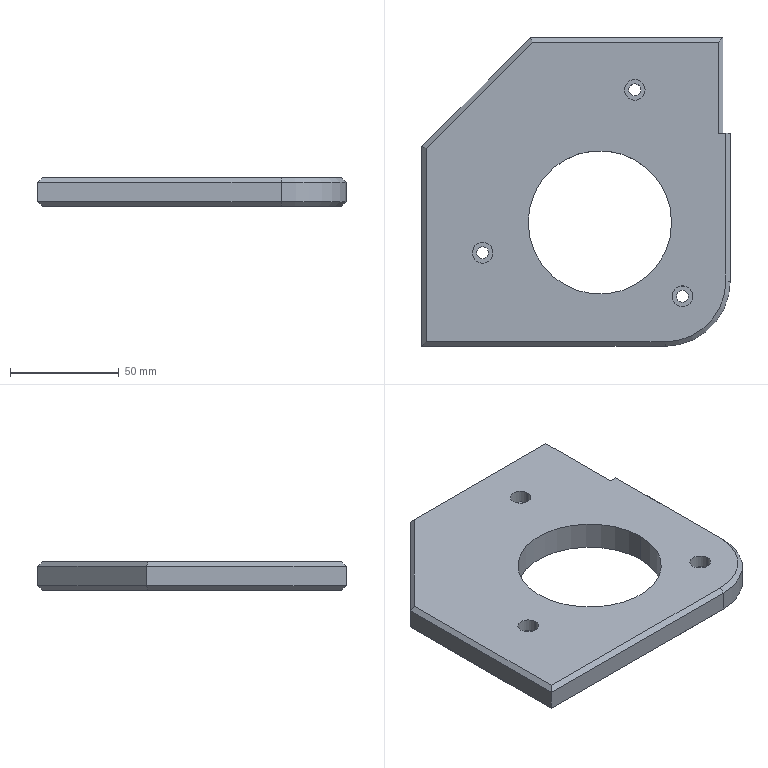Part | Creo | 1 solid | 41 faces | box 142 x 142 x 13 mm | volume 193049 mm3 | plane 24 | cylinder 15 | cone 2 | commonest cylinder face diameters 5.5 x6 9.5 x6 66 x2 60 x1
STEP:
#1=CARTESIAN_POINT('',(-313.,234.995,-24.));
#2=VERTEX_POINT('',#1);
#3=CARTESIAN_POINT('',(-203.,234.995,-24.));
#4=VERTEX_POINT('',#3);
#5=CARTESIAN_POINT('',(-313.,234.995,-24.));
#6=DIRECTION('',(1.,0.,0.));
#7=VECTOR('',#6,110.);
#8=LINE('',#5,#7);
#9=EDGE_CURVE('',#2,#4,#8,.T.);
#10=ORIENTED_EDGE('',*,*,#9,.T.);
#11=CARTESIAN_POINT('',(-175.,262.995,-24.));
#12=VERTEX_POINT('',#11);
#13=CARTESIAN_POINT('',(-203.,262.995,-24.));
#14=DIRECTION('',(0.,0.,-1.));
#15=DIRECTION('',(1.,0.,0.));
#16=AXIS2_PLACEMENT_3D('',#13,#14,#15);
#17=CIRCLE('',#16,28.);
#18=EDGE_CURVE('',#12,#4,#17,.T.);
#19=ORIENTED_EDGE('',*,*,#18,.F.);
#20=CARTESIAN_POINT('',(-175.,330.995,-24.));
#21=VERTEX_POINT('',#20);
#22=CARTESIAN_POINT('',(-175.,262.995,-24.));
#23=DIRECTION('',(0.,1.,0.));
#24=VECTOR('',#23,68.);
#25=LINE('',#22,#24);
#26=EDGE_CURVE('',#12,#21,#25,.T.);
#27=ORIENTED_EDGE('',*,*,#26,.T.);
#28=CARTESIAN_POINT('',(-178.5,330.995,-24.));
#29=VERTEX_POINT('',#28);
#30=CARTESIAN_POINT('',(-175.,330.995,-24.));
#31=DIRECTION('',(-1.,0.,0.));
#32=VECTOR('',#31,3.5);
#33=LINE('',#30,#32);
#34=EDGE_CURVE('',#21,#29,#33,.T.);
#35=ORIENTED_EDGE('',*,*,#34,.T.);
#36=CARTESIAN_POINT('',(-178.5,372.995,-24.));
#37=VERTEX_POINT('',#36);
#38=CARTESIAN_POINT('',(-178.5,330.995,-24.));
#39=DIRECTION('',(0.,1.,0.));
#40=VECTOR('',#39,42.);
#41=LINE('',#38,#40);
#42=EDGE_CURVE('',#29,#37,#41,.T.);
#43=ORIENTED_EDGE('',*,*,#42,.T.);
#44=CARTESIAN_POINT('',(-264.172,372.995,-24.));
#45=VERTEX_POINT('',#44);
#46=CARTESIAN_POINT('',(-178.5,372.995,-24.));
#47=DIRECTION('',(-1.,0.,0.));
#48=VECTOR('',#47,85.672);
#49=LINE('',#46,#48);
#50=EDGE_CURVE('',#37,#45,#49,.T.);
#51=ORIENTED_EDGE('',*,*,#50,.T.);
#52=CARTESIAN_POINT('',(-313.,324.167,-24.));
#53=VERTEX_POINT('',#52);
#54=CARTESIAN_POINT('',(-313.,324.167,-24.));
#55=DIRECTION('',(0.7071,0.7071,0.));
#56=VECTOR('',#55,69.054);
#57=LINE('',#54,#56);
#58=EDGE_CURVE('',#53,#45,#57,.T.);
#59=ORIENTED_EDGE('',*,*,#58,.F.);
#60=CARTESIAN_POINT('',(-313.,324.167,-24.));
#61=DIRECTION('',(0.,-1.,0.));
#62=VECTOR('',#61,89.172);
#63=LINE('',#60,#62);
#64=EDGE_CURVE('',#53,#2,#63,.T.);
#65=ORIENTED_EDGE('',*,*,#64,.T.);
#66=EDGE_LOOP('',(#10,#19,#27,#35,#43,#51,#59,#65));
#67=FACE_OUTER_BOUND('',#66,.F.);
#68=CARTESIAN_POINT('',(-289.75,276.,-24.));
#69=VERTEX_POINT('',#68);
#70=CARTESIAN_POINT('',(-284.25,276.,-24.));
#71=VERTEX_POINT('',#70);
#72=CARTESIAN_POINT('',(-287.,276.,-24.));
#73=DIRECTION('',(0.,0.,1.));
#74=DIRECTION('',(-1.,0.,0.));
#75=AXIS2_PLACEMENT_3D('',#72,#73,#74);
#76=CIRCLE('',#75,2.75);
#77=EDGE_CURVE('',#69,#71,#76,.T.);
#78=ORIENTED_EDGE('',*,*,#77,.F.);
#79=CARTESIAN_POINT('',(-287.,276.,-24.));
#80=DIRECTION('',(0.,0.,1.));
#81=DIRECTION('',(1.,0.,0.));
#82=AXIS2_PLACEMENT_3D('',#79,#80,#81);
#83=CIRCLE('',#82,2.75);
#84=EDGE_CURVE('',#71,#69,#83,.T.);
#85=ORIENTED_EDGE('',*,*,#84,.F.);
#86=EDGE_LOOP('',(#78,#85));
#87=FACE_BOUND('',#86,.F.);
#88=CARTESIAN_POINT('',(-219.699,351.,-24.));
#89=VERTEX_POINT('',#88);
#90=CARTESIAN_POINT('',(-214.199,351.,-24.));
#91=VERTEX_POINT('',#90);
#92=CARTESIAN_POINT('',(-216.949,351.,-24.));
#93=DIRECTION('',(0.,0.,1.));
#94=DIRECTION('',(-1.,0.,0.));
#95=AXIS2_PLACEMENT_3D('',#92,#93,#94);
#96=CIRCLE('',#95,2.75);
#97=EDGE_CURVE('',#89,#91,#96,.T.);
#98=ORIENTED_EDGE('',*,*,#97,.F.);
#99=CARTESIAN_POINT('',(-216.949,351.,-24.));
#100=DIRECTION('',(0.,0.,1.));
#101=DIRECTION('',(1.,0.,0.));
#102=AXIS2_PLACEMENT_3D('',#99,#100,#101);
#103=CIRCLE('',#102,2.75);
#104=EDGE_CURVE('',#91,#89,#103,.T.);
#105=ORIENTED_EDGE('',*,*,#104,.F.);
#106=EDGE_LOOP('',(#98,#105));
#107=FACE_BOUND('',#106,.F.);
#108=CARTESIAN_POINT('',(-197.75,256.,-24.));
#109=VERTEX_POINT('',#108);
#110=CARTESIAN_POINT('',(-192.25,256.,-24.));
#111=VERTEX_POINT('',#110);
#112=CARTESIAN_POINT('',(-195.,256.,-24.));
#113=DIRECTION('',(0.,0.,1.));
#114=DIRECTION('',(-1.,0.,0.));
#115=AXIS2_PLACEMENT_3D('',#112,#113,#114);
#116=CIRCLE('',#115,2.75);
#117=EDGE_CURVE('',#109,#111,#116,.T.);
#118=ORIENTED_EDGE('',*,*,#117,.F.);
#119=CARTESIAN_POINT('',(-195.,256.,-24.));
#120=DIRECTION('',(0.,0.,1.));
#121=DIRECTION('',(1.,0.,0.));
#122=AXIS2_PLACEMENT_3D('',#119,#120,#121);
#123=CIRCLE('',#122,2.75);
#124=EDGE_CURVE('',#111,#109,#123,.T.);
#125=ORIENTED_EDGE('',*,*,#124,.F.);
#126=EDGE_LOOP('',(#118,#125));
#127=FACE_BOUND('',#126,.F.);
#128=CARTESIAN_POINT('',(-266.,289.995,-24.));
#129=VERTEX_POINT('',#128);
#130=CARTESIAN_POINT('',(-200.,289.995,-24.));
#131=VERTEX_POINT('',#130);
#132=CARTESIAN_POINT('',(-233.,289.995,-24.));
#133=DIRECTION('',(0.,0.,1.));
#134=DIRECTION('',(-1.,0.,0.));
#135=AXIS2_PLACEMENT_3D('',#132,#133,#134);
#136=CIRCLE('',#135,33.);
#137=EDGE_CURVE('',#129,#131,#136,.T.);
#138=ORIENTED_EDGE('',*,*,#137,.F.);
#139=CARTESIAN_POINT('',(-233.,289.995,-24.));
#140=DIRECTION('',(0.,0.,1.));
#141=DIRECTION('',(1.,0.,0.));
#142=AXIS2_PLACEMENT_3D('',#139,#140,#141);
#143=CIRCLE('',#142,33.);
#144=EDGE_CURVE('',#131,#129,#143,.T.);
#145=ORIENTED_EDGE('',*,*,#144,.F.);
#146=EDGE_LOOP('',(#138,#145));
#147=FACE_BOUND('',#146,.F.);
#148=CARTESIAN_POINT('',(-223.,300.495,-24.));
#149=DIRECTION('',(0.,0.,-1.));
#150=DIRECTION('',(-1.,0.,0.));
#151=AXIS2_PLACEMENT_3D('',#148,#149,#150);
#152=PLANE('',#151);
#153=ADVANCED_FACE('',(#67,#87,#107,#127,#147),#152,.T.);
#154=ORIENTED_EDGE('',*,*,#117,.T.);
#155=CARTESIAN_POINT('',(-192.25,256.,-17.));
#156=VERTEX_POINT('',#155);
#157=CARTESIAN_POINT('',(-192.25,256.,-24.));
#158=DIRECTION('',(0.,0.,1.));
#159=VECTOR('',#158,7.);
#160=LINE('',#157,#159);
#161=EDGE_CURVE('',#111,#156,#160,.T.);
#162=ORIENTED_EDGE('',*,*,#161,.T.);
#163=CARTESIAN_POINT('',(-197.75,256.,-17.));
#164=VERTEX_POINT('',#163);
#165=CARTESIAN_POINT('',(-195.,256.,-17.));
#166=DIRECTION('',(0.,0.,-1.));
#167=DIRECTION('',(1.,0.,0.));
#168=AXIS2_PLACEMENT_3D('',#165,#166,#167);
#169=CIRCLE('',#168,2.75);
#170=EDGE_CURVE('',#156,#164,#169,.T.);
#171=ORIENTED_EDGE('',*,*,#170,.T.);
#172=CARTESIAN_POINT('',(-197.75,256.,-24.));
#173=DIRECTION('',(0.,0.,1.));
#174=VECTOR('',#173,7.);
#175=LINE('',#172,#174);
#176=EDGE_CURVE('',#109,#164,#175,.T.);
#177=ORIENTED_EDGE('',*,*,#176,.F.);
#178=EDGE_LOOP('',(#154,#162,#171,#177));
#179=FACE_OUTER_BOUND('',#178,.F.);
#180=CARTESIAN_POINT('',(-195.,256.,-11.));
#181=DIRECTION('',(0.,0.,1.));
#182=DIRECTION('',(1.,0.,0.));
#183=AXIS2_PLACEMENT_3D('',#180,#181,#182);
#184=CYLINDRICAL_SURFACE('',#183,2.75);
#185=ADVANCED_FACE('',(#179),#184,.F.);
#186=ORIENTED_EDGE('',*,*,#124,.T.);
#187=ORIENTED_EDGE('',*,*,#176,.T.);
#188=CARTESIAN_POINT('',(-195.,256.,-17.));
#189=DIRECTION('',(0.,0.,-1.));
#190=DIRECTION('',(-1.,0.,0.));
#191=AXIS2_PLACEMENT_3D('',#188,#189,#190);
#192=CIRCLE('',#191,2.75);
#193=EDGE_CURVE('',#164,#156,#192,.T.);
#194=ORIENTED_EDGE('',*,*,#193,.T.);
#195=ORIENTED_EDGE('',*,*,#161,.F.);
#196=EDGE_LOOP('',(#186,#187,#194,#195));
#197=FACE_OUTER_BOUND('',#196,.F.);
#198=CARTESIAN_POINT('',(-195.,256.,-11.));
#199=DIRECTION('',(0.,0.,1.));
#200=DIRECTION('',(1.,0.,0.));
#201=AXIS2_PLACEMENT_3D('',#198,#199,#200);
#202=CYLINDRICAL_SURFACE('',#201,2.75);
#203=ADVANCED_FACE('',(#197),#202,.F.);
#204=CARTESIAN_POINT('',(-190.25,256.,-17.));
#205=VERTEX_POINT('',#204);
#206=CARTESIAN_POINT('',(-199.75,256.,-17.));
#207=VERTEX_POINT('',#206);
#208=CARTESIAN_POINT('',(-195.,256.,-17.));
#209=DIRECTION('',(0.,0.,1.));
#210=DIRECTION('',(1.,0.,0.));
#211=AXIS2_PLACEMENT_3D('',#208,#209,#210);
#212=CIRCLE('',#211,4.75);
#213=EDGE_CURVE('',#205,#207,#212,.T.);
#214=ORIENTED_EDGE('',*,*,#213,.F.);
#215=CARTESIAN_POINT('',(-195.,256.,-17.));
#216=DIRECTION('',(0.,0.,1.));
#217=DIRECTION('',(-1.,0.,0.));
#218=AXIS2_PLACEMENT_3D('',#215,#216,#217);
#219=CIRCLE('',#218,4.75);
#220=EDGE_CURVE('',#207,#205,#219,.T.);
#221=ORIENTED_EDGE('',*,*,#220,.F.);
#222=EDGE_LOOP('',(#214,#221));
#223=FACE_OUTER_BOUND('',#222,.F.);
#224=ORIENTED_EDGE('',*,*,#170,.F.);
#225=ORIENTED_EDGE('',*,*,#193,.F.);
#226=EDGE_LOOP('',(#224,#225));
#227=FACE_BOUND('',#226,.F.);
#228=CARTESIAN_POINT('',(-195.,260.75,-17.));
#229=DIRECTION('',(0.,0.,-1.));
#230=DIRECTION('',(-1.,0.,0.));
#231=AXIS2_PLACEMENT_3D('',#228,#229,#230);
#232=PLANE('',#231);
#233=ADVANCED_FACE('',(#223,#227),#232,.F.);
#234=ORIENTED_EDGE('',*,*,#213,.T.);
#235=CARTESIAN_POINT('',(-199.75,256.,-11.));
#236=VERTEX_POINT('',#235);
#237=CARTESIAN_POINT('',(-199.75,256.,-17.));
#238=DIRECTION('',(0.,0.,1.));
#239=VECTOR('',#238,6.);
#240=LINE('',#237,#239);
#241=EDGE_CURVE('',#207,#236,#240,.T.);
#242=ORIENTED_EDGE('',*,*,#241,.T.);
#243=CARTESIAN_POINT('',(-190.25,256.,-11.));
#244=VERTEX_POINT('',#243);
#245=CARTESIAN_POINT('',(-195.,256.,-11.));
#246=DIRECTION('',(0.,0.,-1.));
#247=DIRECTION('',(-1.,0.,0.));
#248=AXIS2_PLACEMENT_3D('',#245,#246,#247);
#249=CIRCLE('',#248,4.75);
#250=EDGE_CURVE('',#236,#244,#249,.T.);
#251=ORIENTED_EDGE('',*,*,#250,.T.);
#252=CARTESIAN_POINT('',(-190.25,256.,-17.));
#253=DIRECTION('',(0.,0.,1.));
#254=VECTOR('',#253,6.);
#255=LINE('',#252,#254);
#256=EDGE_CURVE('',#205,#244,#255,.T.);
#257=ORIENTED_EDGE('',*,*,#256,.F.);
#258=EDGE_LOOP('',(#234,#242,#251,#257));
#259=FACE_OUTER_BOUND('',#258,.F.);
#260=CARTESIAN_POINT('',(-195.,256.,-11.));
#261=DIRECTION('',(0.,0.,1.));
#262=DIRECTION('',(1.,0.,0.));
#263=AXIS2_PLACEMENT_3D('',#260,#261,#262);
#264=CYLINDRICAL_SURFACE('',#263,4.75);
#265=ADVANCED_FACE('',(#259),#264,.F.);
#266=ORIENTED_EDGE('',*,*,#220,.T.);
#267=ORIENTED_EDGE('',*,*,#256,.T.);
#268=CARTESIAN_POINT('',(-195.,256.,-11.));
#269=DIRECTION('',(0.,0.,-1.));
#270=DIRECTION('',(1.,0.,0.));
#271=AXIS2_PLACEMENT_3D('',#268,#269,#270);
#272=CIRCLE('',#271,4.75);
#273=EDGE_CURVE('',#244,#236,#272,.T.);
#274=ORIENTED_EDGE('',*,*,#273,.T.);
#275=ORIENTED_EDGE('',*,*,#241,.F.);
#276=EDGE_LOOP('',(#266,#267,#274,#275));
#277=FACE_OUTER_BOUND('',#276,.F.);
#278=CARTESIAN_POINT('',(-195.,256.,-11.));
#279=DIRECTION('',(0.,0.,1.));
#280=DIRECTION('',(1.,0.,0.));
#281=AXIS2_PLACEMENT_3D('',#278,#279,#280);
#282=CYLINDRICAL_SURFACE('',#281,4.75);
#283=ADVANCED_FACE('',(#277),#282,.F.);
#284=CARTESIAN_POINT('',(-178.5,330.995,-11.));
#285=VERTEX_POINT('',#284);
#286=CARTESIAN_POINT('',(-175.,330.995,-11.));
#287=VERTEX_POINT('',#286);
#288=CARTESIAN_POINT('',(-178.5,330.995,-11.));
#289=DIRECTION('',(1.,0.,0.));
#290=VECTOR('',#289,3.5);
#291=LINE('',#288,#290);
#292=EDGE_CURVE('',#285,#287,#291,.T.);
#293=ORIENTED_EDGE('',*,*,#292,.T.);
#294=CARTESIAN_POINT('',(-175.,262.995,-11.));
#295=VERTEX_POINT('',#294);
#296=CARTESIAN_POINT('',(-175.,330.995,-11.));
#297=DIRECTION('',(0.,-1.,0.));
#298=VECTOR('',#297,68.);
#299=LINE('',#296,#298);
#300=EDGE_CURVE('',#287,#295,#299,.T.);
#301=ORIENTED_EDGE('',*,*,#300,.T.);
#302=CARTESIAN_POINT('',(-203.,234.995,-11.));
#303=VERTEX_POINT('',#302);
#304=CARTESIAN_POINT('',(-203.,262.995,-11.));
#305=DIRECTION('',(0.,0.,1.));
#306=DIRECTION('',(0.,-1.,0.));
#307=AXIS2_PLACEMENT_3D('',#304,#305,#306);
#308=CIRCLE('',#307,28.);
#309=EDGE_CURVE('',#303,#295,#308,.T.);
#310=ORIENTED_EDGE('',*,*,#309,.F.);
#311=CARTESIAN_POINT('',(-313.,234.995,-11.));
#312=VERTEX_POINT('',#311);
#313=CARTESIAN_POINT('',(-203.,234.995,-11.));
#314=DIRECTION('',(-1.,0.,0.));
#315=VECTOR('',#314,110.);
#316=LINE('',#313,#315);
#317=EDGE_CURVE('',#303,#312,#316,.T.);
#318=ORIENTED_EDGE('',*,*,#317,.T.);
#319=CARTESIAN_POINT('',(-313.,324.167,-11.));
#320=VERTEX_POINT('',#319);
#321=CARTESIAN_POINT('',(-313.,234.995,-11.));
#322=DIRECTION('',(0.,1.,0.));
#323=VECTOR('',#322,89.172);
#324=LINE('',#321,#323);
#325=EDGE_CURVE('',#312,#320,#324,.T.);
#326=ORIENTED_EDGE('',*,*,#325,.T.);
#327=CARTESIAN_POINT('',(-264.172,372.995,-11.));
#328=VERTEX_POINT('',#327);
#329=CARTESIAN_POINT('',(-264.172,372.995,-11.));
#330=DIRECTION('',(-0.7071,-0.7071,0.));
#331=VECTOR('',#330,69.054);
#332=LINE('',#329,#331);
#333=EDGE_CURVE('',#328,#320,#332,.T.);
#334=ORIENTED_EDGE('',*,*,#333,.F.);
#335=CARTESIAN_POINT('',(-178.5,372.995,-11.));
#336=VERTEX_POINT('',#335);
#337=CARTESIAN_POINT('',(-264.172,372.995,-11.));
#338=DIRECTION('',(1.,0.,0.));
#339=VECTOR('',#338,85.672);
#340=LINE('',#337,#339);
#341=EDGE_CURVE('',#328,#336,#340,.T.);
#342=ORIENTED_EDGE('',*,*,#341,.T.);
#343=CARTESIAN_POINT('',(-178.5,372.995,-11.));
#344=DIRECTION('',(0.,-1.,0.));
#345=VECTOR('',#344,42.);
#346=LINE('',#343,#345);
#347=EDGE_CURVE('',#336,#285,#346,.T.);
#348=ORIENTED_EDGE('',*,*,#347,.T.);
#349=EDGE_LOOP('',(#293,#301,#310,#318,#326,#334,#342,#348));
#350=FACE_OUTER_BOUND('',#349,.F.);
#351=ORIENTED_EDGE('',*,*,#273,.F.);
#352=ORIENTED_EDGE('',*,*,#250,.F.);
#353=EDGE_LOOP('',(#351,#352));
#354=FACE_BOUND('',#353,.F.);
#355=CARTESIAN_POINT('',(-282.25,276.,-11.));
#356=VERTEX_POINT('',#355);
#357=CARTESIAN_POINT('',(-291.75,276.,-11.));
#358=VERTEX_POINT('',#357);
#359=CARTESIAN_POINT('',(-287.,276.,-11.));
#360=DIRECTION('',(0.,0.,-1.));
#361=DIRECTION('',(1.,0.,0.));
#362=AXIS2_PLACEMENT_3D('',#359,#360,#361);
#363=CIRCLE('',#362,4.75);
#364=EDGE_CURVE('',#356,#358,#363,.T.);
#365=ORIENTED_EDGE('',*,*,#364,.F.);
#366=CARTESIAN_POINT('',(-287.,276.,-11.));
#367=DIRECTION('',(0.,0.,-1.));
#368=DIRECTION('',(-1.,0.,0.));
#369=AXIS2_PLACEMENT_3D('',#366,#367,#368);
#370=CIRCLE('',#369,4.75);
#371=EDGE_CURVE('',#358,#356,#370,.T.);
#372=ORIENTED_EDGE('',*,*,#371,.F.);
#373=EDGE_LOOP('',(#365,#372));
#374=FACE_BOUND('',#373,.F.);
#375=CARTESIAN_POINT('',(-212.199,351.,-11.));
#376=VERTEX_POINT('',#375);
#377=CARTESIAN_POINT('',(-221.699,351.,-11.));
#378=VERTEX_POINT('',#377);
#379=CARTESIAN_POINT('',(-216.949,351.,-11.));
#380=DIRECTION('',(0.,0.,-1.));
#381=DIRECTION('',(1.,0.,0.));
#382=AXIS2_PLACEMENT_3D('',#379,#380,#381);
#383=CIRCLE('',#382,4.75);
#384=EDGE_CURVE('',#376,#378,#383,.T.);
#385=ORIENTED_EDGE('',*,*,#384,.F.);
#386=CARTESIAN_POINT('',(-216.949,351.,-11.));
#387=DIRECTION('',(0.,0.,-1.));
#388=DIRECTION('',(-1.,0.,0.));
#389=AXIS2_PLACEMENT_3D('',#386,#387,#388);
#390=CIRCLE('',#389,4.75);
#391=EDGE_CURVE('',#378,#376,#390,.T.);
#392=ORIENTED_EDGE('',*,*,#391,.F.);
#393=EDGE_LOOP('',(#385,#392));
#394=FACE_BOUND('',#393,.F.);
#395=CARTESIAN_POINT('',(-200.,289.995,-11.));
#396=VERTEX_POINT('',#395);
#397=CARTESIAN_POINT('',(-266.,289.995,-11.));
#398=VERTEX_POINT('',#397);
#399=CARTESIAN_POINT('',(-233.,289.995,-11.));
#400=DIRECTION('',(0.,0.,-1.));
#401=DIRECTION('',(1.,0.,0.));
#402=AXIS2_PLACEMENT_3D('',#399,#400,#401);
#403=CIRCLE('',#402,33.);
#404=EDGE_CURVE('',#396,#398,#403,.T.);
#405=ORIENTED_EDGE('',*,*,#404,.F.);
#406=CARTESIAN_POINT('',(-233.,289.995,-11.));
#407=DIRECTION('',(0.,0.,-1.));
#408=DIRECTION('',(-1.,0.,0.));
#409=AXIS2_PLACEMENT_3D('',#406,#407,#408);
#410=CIRCLE('',#409,33.);
#411=EDGE_CURVE('',#398,#396,#410,.T.);
#412=ORIENTED_EDGE('',*,*,#411,.F.);
#413=EDGE_LOOP('',(#405,#412));
#414=FACE_BOUND('',#413,.F.);
#415=CARTESIAN_POINT('',(-223.,300.495,-11.));
#416=DIRECTION('',(0.,0.,1.));
#417=DIRECTION('',(1.,0.,0.));
#418=AXIS2_PLACEMENT_3D('',#415,#416,#417);
#419=PLANE('',#418);
#420=ADVANCED_FACE('',(#350,#354,#374,#394,#414),#419,.T.);
#421=CARTESIAN_POINT('',(-173.,330.995,-13.));
#422=VERTEX_POINT('',#421);
#423=CARTESIAN_POINT('',(-173.,330.995,-22.));
#424=VERTEX_POINT('',#423);
#425=CARTESIAN_POINT('',(-173.,330.995,-13.));
#426=DIRECTION('',(0.,0.,-1.));
#427=VECTOR('',#426,9.);
#428=LINE('',#425,#427);
#429=EDGE_CURVE('',#422,#424,#428,.T.);
#430=ORIENTED_EDGE('',*,*,#429,.F.);
#431=CARTESIAN_POINT('',(-175.,330.995,-11.));
#432=DIRECTION('',(0.7071,0.,-0.7071));
#433=VECTOR('',#432,2.828);
#434=LINE('',#431,#433);
#435=EDGE_CURVE('',#287,#422,#434,.T.);
#436=ORIENTED_EDGE('',*,*,#435,.F.);
#437=ORIENTED_EDGE('',*,*,#292,.F.);
#438=CARTESIAN_POINT('',(-176.5,330.995,-13.));
#439=VERTEX_POINT('',#438);
#440=CARTESIAN_POINT('',(-176.5,330.995,-13.));
#441=DIRECTION('',(-0.7071,0.,0.7071));
#442=VECTOR('',#441,2.828);
#443=LINE('',#440,#442);
#444=EDGE_CURVE('',#439,#285,#443,.T.);
#445=ORIENTED_EDGE('',*,*,#444,.F.);
#446=CARTESIAN_POINT('',(-176.5,330.995,-22.));
#447=VERTEX_POINT('',#446);
#448=CARTESIAN_POINT('',(-176.5,330.995,-13.));
#449=DIRECTION('',(0.,0.,-1.));
#450=VECTOR('',#449,9.);
#451=LINE('',#448,#450);
#452=EDGE_CURVE('',#439,#447,#451,.T.);
#453=ORIENTED_EDGE('',*,*,#452,.T.);
#454=CARTESIAN_POINT('',(-178.5,330.995,-24.));
#455=DIRECTION('',(0.7071,0.,0.7071));
#456=VECTOR('',#455,2.828);
#457=LINE('',#454,#456);
#458=EDGE_CURVE('',#29,#447,#457,.T.);
#459=ORIENTED_EDGE('',*,*,#458,.F.);
#460=ORIENTED_EDGE('',*,*,#34,.F.);
#461=CARTESIAN_POINT('',(-173.,330.995,-22.));
#462=DIRECTION('',(-0.7071,0.,-0.7071));
#463=VECTOR('',#462,2.828);
#464=LINE('',#461,#463);
#465=EDGE_CURVE('',#424,#21,#464,.T.);
#466=ORIENTED_EDGE('',*,*,#465,.F.);
#467=EDGE_LOOP('',(#430,#436,#437,#445,#453,#459,#460,#466));
#468=FACE_OUTER_BOUND('',#467,.F.);
#469=CARTESIAN_POINT('',(-155.,330.995,-1.));
#470=DIRECTION('',(0.,1.,0.));
#471=DIRECTION('',(-1.,0.,0.));
#472=AXIS2_PLACEMENT_3D('',#469,#470,#471);
#473=PLANE('',#472);
#474=ADVANCED_FACE('',(#468),#473,.T.);
#475=CARTESIAN_POINT('',(-173.,262.995,-22.));
#476=VERTEX_POINT('',#475);
#477=CARTESIAN_POINT('',(-173.,262.995,-13.));
#478=VERTEX_POINT('',#477);
#479=CARTESIAN_POINT('',(-173.,262.995,-22.));
#480=DIRECTION('',(0.,0.,1.));
#481=VECTOR('',#480,9.);
#482=LINE('',#479,#481);
#483=EDGE_CURVE('',#476,#478,#482,.T.);
#484=ORIENTED_EDGE('',*,*,#483,.T.);
#485=CARTESIAN_POINT('',(-173.,262.995,-13.));
#486=DIRECTION('',(0.,1.,0.));
#487=VECTOR('',#486,68.);
#488=LINE('',#485,#487);
#489=EDGE_CURVE('',#478,#422,#488,.T.);
#490=ORIENTED_EDGE('',*,*,#489,.T.);
#491=ORIENTED_EDGE('',*,*,#429,.T.);
#492=CARTESIAN_POINT('',(-173.,330.995,-22.));
#493=DIRECTION('',(0.,-1.,0.));
#494=VECTOR('',#493,68.);
#495=LINE('',#492,#494);
#496=EDGE_CURVE('',#424,#476,#495,.T.);
#497=ORIENTED_EDGE('',*,*,#496,.T.);
#498=EDGE_LOOP('',(#484,#490,#491,#497));
#499=FACE_OUTER_BOUND('',#498,.F.);
#500=CARTESIAN_POINT('',(-173.,-2.005,-23.));
#501=DIRECTION('',(-1.,0.,0.));
#502=DIRECTION('',(0.,1.,0.));
#503=AXIS2_PLACEMENT_3D('',#500,#501,#502);
#504=PLANE('',#503);
#505=ADVANCED_FACE('',(#499),#504,.F.);
#506=CARTESIAN_POINT('',(-203.,232.995,-13.));
#507=VERTEX_POINT('',#506);
#508=CARTESIAN_POINT('',(-203.,232.995,-22.));
#509=VERTEX_POINT('',#508);
#510=CARTESIAN_POINT('',(-203.,232.995,-13.));
#511=DIRECTION('',(0.,0.,-1.));
#512=VECTOR('',#511,9.);
#513=LINE('',#510,#512);
#514=EDGE_CURVE('',#507,#509,#513,.T.);
#515=ORIENTED_EDGE('',*,*,#514,.F.);
#516=CARTESIAN_POINT('',(-203.,262.995,-13.));
#517=DIRECTION('',(0.,0.,1.));
#518=DIRECTION('',(0.,-1.,0.));
#519=AXIS2_PLACEMENT_3D('',#516,#517,#518);
#520=CIRCLE('',#519,30.);
#521=EDGE_CURVE('',#507,#478,#520,.T.);
#522=ORIENTED_EDGE('',*,*,#521,.T.);
#523=ORIENTED_EDGE('',*,*,#483,.F.);
#524=CARTESIAN_POINT('',(-203.,262.995,-22.));
#525=DIRECTION('',(0.,0.,-1.));
#526=DIRECTION('',(1.,0.,0.));
#527=AXIS2_PLACEMENT_3D('',#524,#525,#526);
#528=CIRCLE('',#527,30.);
#529=EDGE_CURVE('',#476,#509,#528,.T.);
#530=ORIENTED_EDGE('',*,*,#529,.T.);
#531=EDGE_LOOP('',(#515,#522,#523,#530));
#532=FACE_OUTER_BOUND('',#531,.F.);
#533=CARTESIAN_POINT('',(-203.,262.995,-12.));
#534=DIRECTION('',(0.,0.,1.));
#535=DIRECTION('',(1.,0.,0.));
#536=AXIS2_PLACEMENT_3D('',#533,#534,#535);
#537=CYLINDRICAL_SURFACE('',#536,30.);
#538=ADVANCED_FACE('',(#532),#537,.T.);
#539=CARTESIAN_POINT('',(-315.,232.995,-22.));
#540=VERTEX_POINT('',#539);
#541=CARTESIAN_POINT('',(-315.,232.995,-13.));
#542=VERTEX_POINT('',#541);
#543=CARTESIAN_POINT('',(-315.,232.995,-22.));
#544=DIRECTION('',(0.,0.,1.));
#545=VECTOR('',#544,9.);
#546=LINE('',#543,#545);
#547=EDGE_CURVE('',#540,#542,#546,.T.);
#548=ORIENTED_EDGE('',*,*,#547,.T.);
#549=CARTESIAN_POINT('',(-315.,232.995,-13.));
#550=DIRECTION('',(1.,0.,0.));
#551=VECTOR('',#550,112.);
#552=LINE('',#549,#551);
#553=EDGE_CURVE('',#542,#507,#552,.T.);
#554=ORIENTED_EDGE('',*,*,#553,.T.);
#555=ORIENTED_EDGE('',*,*,#514,.T.);
#556=CARTESIAN_POINT('',(-203.,232.995,-22.));
#557=DIRECTION('',(-1.,0.,0.));
#558=VECTOR('',#557,112.);
#559=LINE('',#556,#558);
#560=EDGE_CURVE('',#509,#540,#559,.T.);
#561=ORIENTED_EDGE('',*,*,#560,.T.);
#562=EDGE_LOOP('',(#548,#554,#555,#561));
#563=FACE_OUTER_BOUND('',#562,.F.);
#564=CARTESIAN_POINT('',(-223.,232.995,-12.));
#565=DIRECTION('',(0.,-1.,0.));
#566=DIRECTION('',(0.,0.,-1.));
#567=AXIS2_PLACEMENT_3D('',#564,#565,#566);
#568=PLANE('',#567);
#569=ADVANCED_FACE('',(#563),#568,.T.);
#570=CARTESIAN_POINT('',(-315.,324.995,-22.));
#571=VERTEX_POINT('',#570);
#572=CARTESIAN_POINT('',(-315.,324.995,-13.));
#573=VERTEX_POINT('',#572);
#574=CARTESIAN_POINT('',(-315.,324.995,-22.));
#575=DIRECTION('',(0.,0.,1.));
#576=VECTOR('',#575,9.);
#577=LINE('',#574,#576);
#578=EDGE_CURVE('',#571,#573,#577,.T.);
#579=ORIENTED_EDGE('',*,*,#578,.T.);
#580=CARTESIAN_POINT('',(-315.,324.995,-13.));
#581=DIRECTION('',(0.,-1.,0.));
#582=VECTOR('',#581,92.);
#583=LINE('',#580,#582);
#584=EDGE_CURVE('',#573,#542,#583,.T.);
#585=ORIENTED_EDGE('',*,*,#584,.T.);
#586=ORIENTED_EDGE('',*,*,#547,.F.);
#587=CARTESIAN_POINT('',(-315.,232.995,-22.));
#588=DIRECTION('',(0.,1.,0.));
#589=VECTOR('',#588,92.);
#590=LINE('',#587,#589);
#591=EDGE_CURVE('',#540,#571,#590,.T.);
#592=ORIENTED_EDGE('',*,*,#591,.T.);
#593=EDGE_LOOP('',(#579,#585,#586,#592));
#594=FACE_OUTER_BOUND('',#593,.F.);
#595=CARTESIAN_POINT('',(-315.,-0.004699,-21.));
#596=DIRECTION('',(1.,0.,0.));
#597=DIRECTION('',(0.,-1.,0.));
#598=AXIS2_PLACEMENT_3D('',#595,#596,#597);
#599=PLANE('',#598);
#600=ADVANCED_FACE('',(#594),#599,.F.);
#601=CARTESIAN_POINT('',(-265.,374.995,-13.));
#602=VERTEX_POINT('',#601);
#603=CARTESIAN_POINT('',(-265.,374.995,-22.));
#604=VERTEX_POINT('',#603);
#605=CARTESIAN_POINT('',(-265.,374.995,-13.));
#606=DIRECTION('',(0.,0.,-1.));
#607=VECTOR('',#606,9.);
#608=LINE('',#605,#607);
#609=EDGE_CURVE('',#602,#604,#608,.T.);
#610=ORIENTED_EDGE('',*,*,#609,.F.);
#611=CARTESIAN_POINT('',(-265.,374.995,-13.));
#612=DIRECTION('',(-0.7071,-0.7071,0.));
#613=VECTOR('',#612,70.711);
#614=LINE('',#611,#613);
#615=EDGE_CURVE('',#602,#573,#614,.T.);
#616=ORIENTED_EDGE('',*,*,#615,.T.);
#617=ORIENTED_EDGE('',*,*,#578,.F.);
#618=CARTESIAN_POINT('',(-315.,324.995,-22.));
#619=DIRECTION('',(0.7071,0.7071,0.));
#620=VECTOR('',#619,70.711);
#621=LINE('',#618,#620);
#622=EDGE_CURVE('',#571,#604,#621,.T.);
#623=ORIENTED_EDGE('',*,*,#622,.T.);
#624=EDGE_LOOP('',(#610,#616,#617,#623));
#625=FACE_OUTER_BOUND('',#624,.F.);
#626=CARTESIAN_POINT('',(-315.,324.995,-21.));
#627=DIRECTION('',(-0.7071,0.7071,0.));
#628=DIRECTION('',(0.,0.,1.));
#629=AXIS2_PLACEMENT_3D('',#626,#627,#628);
#630=PLANE('',#629);
#631=ADVANCED_FACE('',(#625),#630,.T.);
#632=CARTESIAN_POINT('',(-176.5,374.995,-22.));
#633=VERTEX_POINT('',#632);
#634=CARTESIAN_POINT('',(-176.5,374.995,-13.));
#635=VERTEX_POINT('',#634);
#636=CARTESIAN_POINT('',(-176.5,374.995,-22.));
#637=DIRECTION('',(0.,0.,1.));
#638=VECTOR('',#637,9.);
#639=LINE('',#636,#638);
#640=EDGE_CURVE('',#633,#635,#639,.T.);
#641=ORIENTED_EDGE('',*,*,#640,.T.);
#642=CARTESIAN_POINT('',(-176.5,374.995,-13.));
#643=DIRECTION('',(-1.,0.,0.));
#644=VECTOR('',#643,88.5);
#645=LINE('',#642,#644);
#646=EDGE_CURVE('',#635,#602,#645,.T.);
#647=ORIENTED_EDGE('',*,*,#646,.T.);
#648=ORIENTED_EDGE('',*,*,#609,.T.);
#649=CARTESIAN_POINT('',(-265.,374.995,-22.));
#650=DIRECTION('',(1.,0.,0.));
#651=VECTOR('',#650,88.5);
#652=LINE('',#649,#651);
#653=EDGE_CURVE('',#604,#633,#652,.T.);
#654=ORIENTED_EDGE('',*,*,#653,.T.);
#655=EDGE_LOOP('',(#641,#647,#648,#654));
#656=FACE_OUTER_BOUND('',#655,.F.);
#657=CARTESIAN_POINT('',(-265.,374.995,-21.));
#658=DIRECTION('',(0.,1.,0.));
#659=DIRECTION('',(0.,0.,-1.));
#660=AXIS2_PLACEMENT_3D('',#657,#658,#659);
#661=PLANE('',#660);
#662=ADVANCED_FACE('',(#656),#661,.T.);
#663=ORIENTED_EDGE('',*,*,#452,.F.);
#664=CARTESIAN_POINT('',(-176.5,330.995,-13.));
#665=DIRECTION('',(0.,1.,0.));
#666=VECTOR('',#665,44.);
#667=LINE('',#664,#666);
#668=EDGE_CURVE('',#439,#635,#667,.T.);
#669=ORIENTED_EDGE('',*,*,#668,.T.);
#670=ORIENTED_EDGE('',*,*,#640,.F.);
#671=CARTESIAN_POINT('',(-176.5,374.995,-22.));
#672=DIRECTION('',(0.,-1.,0.));
#673=VECTOR('',#672,44.);
#674=LINE('',#671,#673);
#675=EDGE_CURVE('',#633,#447,#674,.T.);
#676=ORIENTED_EDGE('',*,*,#675,.T.);
#677=EDGE_LOOP('',(#663,#669,#670,#676));
#678=FACE_OUTER_BOUND('',#677,.F.);
#679=CARTESIAN_POINT('',(-176.5,393.995,173.076));
#680=DIRECTION('',(-1.,0.,0.));
#681=DIRECTION('',(0.,0.,-1.));
#682=AXIS2_PLACEMENT_3D('',#679,#680,#681);
#683=PLANE('',#682);
#684=ADVANCED_FACE('',(#678),#683,.F.);
#685=ORIENTED_EDGE('',*,*,#444,.T.);
#686=ORIENTED_EDGE('',*,*,#347,.F.);
#687=CARTESIAN_POINT('',(-178.5,372.995,-11.));
#688=DIRECTION('',(0.5774,0.5774,-0.5774));
#689=VECTOR('',#688,3.464);
#690=LINE('',#687,#689);
#691=EDGE_CURVE('',#336,#635,#690,.T.);
#692=ORIENTED_EDGE('',*,*,#691,.T.);
#693=ORIENTED_EDGE('',*,*,#668,.F.);
#694=EDGE_LOOP('',(#685,#686,#692,#693));
#695=FACE_OUTER_BOUND('',#694,.F.);
#696=CARTESIAN_POINT('',(-178.5,300.495,-11.));
#697=DIRECTION('',(0.7071,0.,0.7071));
#698=DIRECTION('',(0.,-1.,0.));
#699=AXIS2_PLACEMENT_3D('',#696,#697,#698);
#700=PLANE('',#699);
#701=ADVANCED_FACE('',(#695),#700,.T.);
#702=CARTESIAN_POINT('',(-264.172,372.995,-11.));
#703=DIRECTION('',(-0.2811,0.6786,-0.6786));
#704=VECTOR('',#703,2.947);
#705=LINE('',#702,#704);
#706=EDGE_CURVE('',#328,#602,#705,.T.);
#707=ORIENTED_EDGE('',*,*,#706,.T.);
#708=ORIENTED_EDGE('',*,*,#646,.F.);
#709=ORIENTED_EDGE('',*,*,#691,.F.);
#710=ORIENTED_EDGE('',*,*,#341,.F.);
#711=EDGE_LOOP('',(#707,#708,#709,#710));
#712=FACE_OUTER_BOUND('',#711,.F.);
#713=CARTESIAN_POINT('',(-223.,372.995,-11.));
#714=DIRECTION('',(0.,-0.7071,-0.7071));
#715=DIRECTION('',(-1.,0.,0.));
#716=AXIS2_PLACEMENT_3D('',#713,#714,#715);
#717=PLANE('',#716);
#718=ADVANCED_FACE('',(#712),#717,.F.);
#719=CARTESIAN_POINT('',(-313.,324.167,-11.));
#720=DIRECTION('',(-0.6786,0.2811,-0.6786));
#721=VECTOR('',#720,2.947);
#722=LINE('',#719,#721);
#723=EDGE_CURVE('',#320,#573,#722,.T.);
#724=ORIENTED_EDGE('',*,*,#723,.T.);
#725=ORIENTED_EDGE('',*,*,#615,.F.);
#726=ORIENTED_EDGE('',*,*,#706,.F.);
#727=ORIENTED_EDGE('',*,*,#333,.T.);
#728=EDGE_LOOP('',(#724,#725,#726,#727));
#729=FACE_OUTER_BOUND('',#728,.F.);
#730=CARTESIAN_POINT('',(-279.836,357.331,-11.));
#731=DIRECTION('',(0.5,-0.5,-0.7071));
#732=DIRECTION('',(-0.7071,-0.7071,0.));
#733=AXIS2_PLACEMENT_3D('',#730,#731,#732);
#734=PLANE('',#733);
#735=ADVANCED_FACE('',(#729),#734,.F.);
#736=CARTESIAN_POINT('',(-313.,234.995,-11.));
#737=DIRECTION('',(-0.5774,-0.5774,-0.5774));
#738=VECTOR('',#737,3.464);
#739=LINE('',#736,#738);
#740=EDGE_CURVE('',#312,#542,#739,.T.);
#741=ORIENTED_EDGE('',*,*,#740,.T.);
#742=ORIENTED_EDGE('',*,*,#584,.F.);
#743=ORIENTED_EDGE('',*,*,#723,.F.);
#744=ORIENTED_EDGE('',*,*,#325,.F.);
#745=EDGE_LOOP('',(#741,#742,#743,#744));
#746=FACE_OUTER_BOUND('',#745,.F.);
#747=CARTESIAN_POINT('',(-313.,300.495,-11.));
#748=DIRECTION('',(-0.7071,0.,0.7071));
#749=DIRECTION('',(0.,1.,0.));
#750=AXIS2_PLACEMENT_3D('',#747,#748,#749);
#751=PLANE('',#750);
#752=ADVANCED_FACE('',(#746),#751,.T.);
#753=CARTESIAN_POINT('',(-203.,234.995,-11.));
#754=DIRECTION('',(0.,-0.7071,-0.7071));
#755=VECTOR('',#754,2.828);
#756=LINE('',#753,#755);
#757=EDGE_CURVE('',#303,#507,#756,.T.);
#758=ORIENTED_EDGE('',*,*,#757,.T.);
#759=ORIENTED_EDGE('',*,*,#553,.F.);
#760=ORIENTED_EDGE('',*,*,#740,.F.);
#761=ORIENTED_EDGE('',*,*,#317,.F.);
#762=EDGE_LOOP('',(#758,#759,#760,#761));
#763=FACE_OUTER_BOUND('',#762,.F.);
#764=CARTESIAN_POINT('',(-223.,234.995,-11.));
#765=DIRECTION('',(0.,0.7071,-0.7071));
#766=DIRECTION('',(1.,0.,0.));
#767=AXIS2_PLACEMENT_3D('',#764,#765,#766);
#768=PLANE('',#767);
#769=ADVANCED_FACE('',(#763),#768,.F.);
#770=CARTESIAN_POINT('',(-173.,262.995,-13.));
#771=DIRECTION('',(-0.7071,0.,0.7071));
#772=VECTOR('',#771,2.828);
#773=LINE('',#770,#772);
#774=EDGE_CURVE('',#478,#295,#773,.T.);
#775=ORIENTED_EDGE('',*,*,#774,.F.);
#776=ORIENTED_EDGE('',*,*,#521,.F.);
#777=ORIENTED_EDGE('',*,*,#757,.F.);
#778=ORIENTED_EDGE('',*,*,#309,.T.);
#779=EDGE_LOOP('',(#775,#776,#777,#778));
#780=FACE_OUTER_BOUND('',#779,.F.);
#781=CARTESIAN_POINT('',(-203.,262.995,-12.));
#782=DIRECTION('',(0.,0.,-1.));
#783=DIRECTION('',(-1.,0.,0.));
#784=AXIS2_PLACEMENT_3D('',#781,#782,#783);
#785=CONICAL_SURFACE('',#784,29.,45.);
#786=ADVANCED_FACE('',(#780),#785,.T.);
#787=ORIENTED_EDGE('',*,*,#435,.T.);
#788=ORIENTED_EDGE('',*,*,#489,.F.);
#789=ORIENTED_EDGE('',*,*,#774,.T.);
#790=ORIENTED_EDGE('',*,*,#300,.F.);
#791=EDGE_LOOP('',(#787,#788,#789,#790));
#792=FACE_OUTER_BOUND('',#791,.F.);
#793=CARTESIAN_POINT('',(-175.,300.495,-11.));
#794=DIRECTION('',(0.7071,0.,0.7071));
#795=DIRECTION('',(0.,-1.,0.));
#796=AXIS2_PLACEMENT_3D('',#793,#794,#795);
#797=PLANE('',#796);
#798=ADVANCED_FACE('',(#792),#797,.T.);
#799=ORIENTED_EDGE('',*,*,#458,.T.);
#800=ORIENTED_EDGE('',*,*,#675,.F.);
#801=CARTESIAN_POINT('',(-178.5,372.995,-24.));
#802=DIRECTION('',(0.5774,0.5774,0.5774));
#803=VECTOR('',#802,3.464);
#804=LINE('',#801,#803);
#805=EDGE_CURVE('',#37,#633,#804,.T.);
#806=ORIENTED_EDGE('',*,*,#805,.F.);
#807=ORIENTED_EDGE('',*,*,#42,.F.);
#808=EDGE_LOOP('',(#799,#800,#806,#807));
#809=FACE_OUTER_BOUND('',#808,.F.);
#810=CARTESIAN_POINT('',(-178.5,300.495,-24.));
#811=DIRECTION('',(0.7071,0.,-0.7071));
#812=DIRECTION('',(0.,1.,0.));
#813=AXIS2_PLACEMENT_3D('',#810,#811,#812);
#814=PLANE('',#813);
#815=ADVANCED_FACE('',(#809),#814,.T.);
#816=ORIENTED_EDGE('',*,*,#805,.T.);
#817=ORIENTED_EDGE('',*,*,#653,.F.);
#818=CARTESIAN_POINT('',(-264.172,372.995,-24.));
#819=DIRECTION('',(-0.2811,0.6786,0.6786));
#820=VECTOR('',#819,2.947);
#821=LINE('',#818,#820);
#822=EDGE_CURVE('',#45,#604,#821,.T.);
#823=ORIENTED_EDGE('',*,*,#822,.F.);
#824=ORIENTED_EDGE('',*,*,#50,.F.);
#825=EDGE_LOOP('',(#816,#817,#823,#824));
#826=FACE_OUTER_BOUND('',#825,.F.);
#827=CARTESIAN_POINT('',(-223.,372.995,-24.));
#828=DIRECTION('',(0.,-0.7071,0.7071));
#829=DIRECTION('',(1.,0.,0.));
#830=AXIS2_PLACEMENT_3D('',#827,#828,#829);
#831=PLANE('',#830);
#832=ADVANCED_FACE('',(#826),#831,.F.);
#833=ORIENTED_EDGE('',*,*,#58,.T.);
#834=ORIENTED_EDGE('',*,*,#822,.T.);
#835=ORIENTED_EDGE('',*,*,#622,.F.);
#836=CARTESIAN_POINT('',(-315.,324.995,-22.));
#837=DIRECTION('',(0.6786,-0.2811,-0.6786));
#838=VECTOR('',#837,2.947);
#839=LINE('',#836,#838);
#840=EDGE_CURVE('',#571,#53,#839,.T.);
#841=ORIENTED_EDGE('',*,*,#840,.T.);
#842=EDGE_LOOP('',(#833,#834,#835,#841));
#843=FACE_OUTER_BOUND('',#842,.F.);
#844=CARTESIAN_POINT('',(-279.836,357.331,-24.));
#845=DIRECTION('',(0.5,-0.5,0.7071));
#846=DIRECTION('',(0.7071,0.7071,0.));
#847=AXIS2_PLACEMENT_3D('',#844,#845,#846);
#848=PLANE('',#847);
#849=ADVANCED_FACE('',(#843),#848,.F.);
#850=CARTESIAN_POINT('',(-313.,234.995,-24.));
#851=DIRECTION('',(-0.5774,-0.5774,0.5774));
#852=VECTOR('',#851,3.464);
#853=LINE('',#850,#852);
#854=EDGE_CURVE('',#2,#540,#853,.T.);
#855=ORIENTED_EDGE('',*,*,#854,.F.);
#856=ORIENTED_EDGE('',*,*,#64,.F.);
#857=ORIENTED_EDGE('',*,*,#840,.F.);
#858=ORIENTED_EDGE('',*,*,#591,.F.);
#859=EDGE_LOOP('',(#855,#856,#857,#858));
#860=FACE_OUTER_BOUND('',#859,.F.);
#861=CARTESIAN_POINT('',(-313.,300.495,-24.));
#862=DIRECTION('',(-0.7071,0.,-0.7071));
#863=DIRECTION('',(0.,-1.,0.));
#864=AXIS2_PLACEMENT_3D('',#861,#862,#863);
#865=PLANE('',#864);
#866=ADVANCED_FACE('',(#860),#865,.T.);
#867=ORIENTED_EDGE('',*,*,#560,.F.);
#868=CARTESIAN_POINT('',(-203.,232.995,-22.));
#869=DIRECTION('',(0.,0.7071,-0.7071));
#870=VECTOR('',#869,2.828);
#871=LINE('',#868,#870);
#872=EDGE_CURVE('',#509,#4,#871,.T.);
#873=ORIENTED_EDGE('',*,*,#872,.T.);
#874=ORIENTED_EDGE('',*,*,#9,.F.);
#875=ORIENTED_EDGE('',*,*,#854,.T.);
#876=EDGE_LOOP('',(#867,#873,#874,#875));
#877=FACE_OUTER_BOUND('',#876,.F.);
#878=CARTESIAN_POINT('',(-223.,234.995,-24.));
#879=DIRECTION('',(0.,0.7071,0.7071));
#880=DIRECTION('',(-1.,0.,0.));
#881=AXIS2_PLACEMENT_3D('',#878,#879,#880);
#882=PLANE('',#881);
#883=ADVANCED_FACE('',(#877),#882,.F.);
#884=CARTESIAN_POINT('',(-175.,262.995,-24.));
#885=DIRECTION('',(0.7071,0.,0.7071));
#886=VECTOR('',#885,2.828);
#887=LINE('',#884,#886);
#888=EDGE_CURVE('',#12,#476,#887,.T.);
#889=ORIENTED_EDGE('',*,*,#888,.F.);
#890=ORIENTED_EDGE('',*,*,#18,.T.);
#891=ORIENTED_EDGE('',*,*,#872,.F.);
#892=ORIENTED_EDGE('',*,*,#529,.F.);
#893=EDGE_LOOP('',(#889,#890,#891,#892));
#894=FACE_OUTER_BOUND('',#893,.F.);
#895=CARTESIAN_POINT('',(-203.,262.995,-23.));
#896=DIRECTION('',(0.,0.,1.));
#897=DIRECTION('',(1.,0.,0.));
#898=AXIS2_PLACEMENT_3D('',#895,#896,#897);
#899=CONICAL_SURFACE('',#898,29.,45.);
#900=ADVANCED_FACE('',(#894),#899,.T.);
#901=ORIENTED_EDGE('',*,*,#465,.T.);
#902=ORIENTED_EDGE('',*,*,#26,.F.);
#903=ORIENTED_EDGE('',*,*,#888,.T.);
#904=ORIENTED_EDGE('',*,*,#496,.F.);
#905=EDGE_LOOP('',(#901,#902,#903,#904));
#906=FACE_OUTER_BOUND('',#905,.F.);
#907=CARTESIAN_POINT('',(-175.,300.495,-24.));
#908=DIRECTION('',(0.7071,0.,-0.7071));
#909=DIRECTION('',(0.,1.,0.));
#910=AXIS2_PLACEMENT_3D('',#907,#908,#909);
#911=PLANE('',#910);
#912=ADVANCED_FACE('',(#906),#911,.T.);
#913=CARTESIAN_POINT('',(-291.75,276.,-17.));
#914=VERTEX_POINT('',#913);
#915=CARTESIAN_POINT('',(-282.25,276.,-17.));
#916=VERTEX_POINT('',#915);
#917=CARTESIAN_POINT('',(-287.,276.,-17.));
#918=DIRECTION('',(0.,0.,1.));
#919=DIRECTION('',(-1.,0.,0.));
#920=AXIS2_PLACEMENT_3D('',#917,#918,#919);
#921=CIRCLE('',#920,4.75);
#922=EDGE_CURVE('',#914,#916,#921,.T.);
#923=ORIENTED_EDGE('',*,*,#922,.T.);
#924=CARTESIAN_POINT('',(-282.25,276.,-17.));
#925=DIRECTION('',(0.,0.,1.));
#926=VECTOR('',#925,6.);
#927=LINE('',#924,#926);
#928=EDGE_CURVE('',#916,#356,#927,.T.);
#929=ORIENTED_EDGE('',*,*,#928,.T.);
#930=ORIENTED_EDGE('',*,*,#364,.T.);
#931=CARTESIAN_POINT('',(-291.75,276.,-17.));
#932=DIRECTION('',(0.,0.,1.));
#933=VECTOR('',#932,6.);
#934=LINE('',#931,#933);
#935=EDGE_CURVE('',#914,#358,#934,.T.);
#936=ORIENTED_EDGE('',*,*,#935,.F.);
#937=EDGE_LOOP('',(#923,#929,#930,#936));
#938=FACE_OUTER_BOUND('',#937,.F.);
#939=CARTESIAN_POINT('',(-287.,276.,-11.));
#940=DIRECTION('',(0.,0.,1.));
#941=DIRECTION('',(1.,0.,0.));
#942=AXIS2_PLACEMENT_3D('',#939,#940,#941);
#943=CYLINDRICAL_SURFACE('',#942,4.75);
#944=ADVANCED_FACE('',(#938),#943,.F.);
#945=CARTESIAN_POINT('',(-287.,276.,-17.));
#946=DIRECTION('',(0.,0.,1.));
#947=DIRECTION('',(1.,0.,0.));
#948=AXIS2_PLACEMENT_3D('',#945,#946,#947);
#949=CIRCLE('',#948,4.75);
#950=EDGE_CURVE('',#916,#914,#949,.T.);
#951=ORIENTED_EDGE('',*,*,#950,.F.);
#952=ORIENTED_EDGE('',*,*,#922,.F.);
#953=EDGE_LOOP('',(#951,#952));
#954=FACE_OUTER_BOUND('',#953,.F.);
#955=CARTESIAN_POINT('',(-284.25,276.,-17.));
#956=VERTEX_POINT('',#955);
#957=CARTESIAN_POINT('',(-289.75,276.,-17.));
#958=VERTEX_POINT('',#957);
#959=CARTESIAN_POINT('',(-287.,276.,-17.));
#960=DIRECTION('',(0.,0.,-1.));
#961=DIRECTION('',(1.,0.,0.));
#962=AXIS2_PLACEMENT_3D('',#959,#960,#961);
#963=CIRCLE('',#962,2.75);
#964=EDGE_CURVE('',#956,#958,#963,.T.);
#965=ORIENTED_EDGE('',*,*,#964,.F.);
#966=CARTESIAN_POINT('',(-287.,276.,-17.));
#967=DIRECTION('',(0.,0.,-1.));
#968=DIRECTION('',(-1.,0.,0.));
#969=AXIS2_PLACEMENT_3D('',#966,#967,#968);
#970=CIRCLE('',#969,2.75);
#971=EDGE_CURVE('',#958,#956,#970,.T.);
#972=ORIENTED_EDGE('',*,*,#971,.F.);
#973=EDGE_LOOP('',(#965,#972));
#974=FACE_BOUND('',#973,.F.);
#975=CARTESIAN_POINT('',(-287.,280.75,-17.));
#976=DIRECTION('',(0.,0.,-1.));
#977=DIRECTION('',(-1.,0.,0.));
#978=AXIS2_PLACEMENT_3D('',#975,#976,#977);
#979=PLANE('',#978);
#980=ADVANCED_FACE('',(#954,#974),#979,.F.);
#981=ORIENTED_EDGE('',*,*,#77,.T.);
#982=CARTESIAN_POINT('',(-284.25,276.,-24.));
#983=DIRECTION('',(0.,0.,1.));
#984=VECTOR('',#983,7.);
#985=LINE('',#982,#984);
#986=EDGE_CURVE('',#71,#956,#985,.T.);
#987=ORIENTED_EDGE('',*,*,#986,.T.);
#988=ORIENTED_EDGE('',*,*,#964,.T.);
#989=CARTESIAN_POINT('',(-289.75,276.,-24.));
#990=DIRECTION('',(0.,0.,1.));
#991=VECTOR('',#990,7.);
#992=LINE('',#989,#991);
#993=EDGE_CURVE('',#69,#958,#992,.T.);
#994=ORIENTED_EDGE('',*,*,#993,.F.);
#995=EDGE_LOOP('',(#981,#987,#988,#994));
#996=FACE_OUTER_BOUND('',#995,.F.);
#997=CARTESIAN_POINT('',(-287.,276.,-11.));
#998=DIRECTION('',(0.,0.,1.));
#999=DIRECTION('',(1.,0.,0.));
#1000=AXIS2_PLACEMENT_3D('',#997,#998,#999);
#1001=CYLINDRICAL_SURFACE('',#1000,2.75);
#1002=ADVANCED_FACE('',(#996),#1001,.F.);
#1003=ORIENTED_EDGE('',*,*,#84,.T.);
#1004=ORIENTED_EDGE('',*,*,#993,.T.);
#1005=ORIENTED_EDGE('',*,*,#971,.T.);
#1006=ORIENTED_EDGE('',*,*,#986,.F.);
#1007=EDGE_LOOP('',(#1003,#1004,#1005,#1006));
#1008=FACE_OUTER_BOUND('',#1007,.F.);
#1009=CARTESIAN_POINT('',(-287.,276.,-11.));
#1010=DIRECTION('',(0.,0.,1.));
#1011=DIRECTION('',(1.,0.,0.));
#1012=AXIS2_PLACEMENT_3D('',#1009,#1010,#1011);
#1013=CYLINDRICAL_SURFACE('',#1012,2.75);
#1014=ADVANCED_FACE('',(#1008),#1013,.F.);
#1015=ORIENTED_EDGE('',*,*,#950,.T.);
#1016=ORIENTED_EDGE('',*,*,#935,.T.);
#1017=ORIENTED_EDGE('',*,*,#371,.T.);
#1018=ORIENTED_EDGE('',*,*,#928,.F.);
#1019=EDGE_LOOP('',(#1015,#1016,#1017,#1018));
#1020=FACE_OUTER_BOUND('',#1019,.F.);
#1021=CARTESIAN_POINT('',(-287.,276.,-11.));
#1022=DIRECTION('',(0.,0.,1.));
#1023=DIRECTION('',(1.,0.,0.));
#1024=AXIS2_PLACEMENT_3D('',#1021,#1022,#1023);
#1025=CYLINDRICAL_SURFACE('',#1024,4.75);
#1026=ADVANCED_FACE('',(#1020),#1025,.F.);
#1027=CARTESIAN_POINT('',(-221.699,351.,-17.));
#1028=VERTEX_POINT('',#1027);
#1029=CARTESIAN_POINT('',(-212.199,351.,-17.));
#1030=VERTEX_POINT('',#1029);
#1031=CARTESIAN_POINT('',(-216.949,351.,-17.));
#1032=DIRECTION('',(0.,0.,1.));
#1033=DIRECTION('',(-1.,0.,0.));
#1034=AXIS2_PLACEMENT_3D('',#1031,#1032,#1033);
#1035=CIRCLE('',#1034,4.75);
#1036=EDGE_CURVE('',#1028,#1030,#1035,.T.);
#1037=ORIENTED_EDGE('',*,*,#1036,.T.);
#1038=CARTESIAN_POINT('',(-212.199,351.,-17.));
#1039=DIRECTION('',(0.,0.,1.));
#1040=VECTOR('',#1039,6.);
#1041=LINE('',#1038,#1040);
#1042=EDGE_CURVE('',#1030,#376,#1041,.T.);
#1043=ORIENTED_EDGE('',*,*,#1042,.T.);
#1044=ORIENTED_EDGE('',*,*,#384,.T.);
#1045=CARTESIAN_POINT('',(-221.699,351.,-17.));
#1046=DIRECTION('',(0.,0.,1.));
#1047=VECTOR('',#1046,6.);
#1048=LINE('',#1045,#1047);
#1049=EDGE_CURVE('',#1028,#378,#1048,.T.);
#1050=ORIENTED_EDGE('',*,*,#1049,.F.);
#1051=EDGE_LOOP('',(#1037,#1043,#1044,#1050));
#1052=FACE_OUTER_BOUND('',#1051,.F.);
#1053=CARTESIAN_POINT('',(-216.949,351.,-11.));
#1054=DIRECTION('',(0.,0.,1.));
#1055=DIRECTION('',(1.,0.,0.));
#1056=AXIS2_PLACEMENT_3D('',#1053,#1054,#1055);
#1057=CYLINDRICAL_SURFACE('',#1056,4.75);
#1058=ADVANCED_FACE('',(#1052),#1057,.F.);
#1059=CARTESIAN_POINT('',(-216.949,351.,-17.));
#1060=DIRECTION('',(0.,0.,1.));
#1061=DIRECTION('',(1.,0.,0.));
#1062=AXIS2_PLACEMENT_3D('',#1059,#1060,#1061);
#1063=CIRCLE('',#1062,4.75);
#1064=EDGE_CURVE('',#1030,#1028,#1063,.T.);
#1065=ORIENTED_EDGE('',*,*,#1064,.F.);
#1066=ORIENTED_EDGE('',*,*,#1036,.F.);
#1067=EDGE_LOOP('',(#1065,#1066));
#1068=FACE_OUTER_BOUND('',#1067,.F.);
#1069=CARTESIAN_POINT('',(-214.199,351.,-17.));
#1070=VERTEX_POINT('',#1069);
#1071=CARTESIAN_POINT('',(-219.699,351.,-17.));
#1072=VERTEX_POINT('',#1071);
#1073=CARTESIAN_POINT('',(-216.949,351.,-17.));
#1074=DIRECTION('',(0.,0.,-1.));
#1075=DIRECTION('',(1.,0.,0.));
#1076=AXIS2_PLACEMENT_3D('',#1073,#1074,#1075);
#1077=CIRCLE('',#1076,2.75);
#1078=EDGE_CURVE('',#1070,#1072,#1077,.T.);
#1079=ORIENTED_EDGE('',*,*,#1078,.F.);
#1080=CARTESIAN_POINT('',(-216.949,351.,-17.));
#1081=DIRECTION('',(0.,0.,-1.));
#1082=DIRECTION('',(-1.,0.,0.));
#1083=AXIS2_PLACEMENT_3D('',#1080,#1081,#1082);
#1084=CIRCLE('',#1083,2.75);
#1085=EDGE_CURVE('',#1072,#1070,#1084,.T.);
#1086=ORIENTED_EDGE('',*,*,#1085,.F.);
#1087=EDGE_LOOP('',(#1079,#1086));
#1088=FACE_BOUND('',#1087,.F.);
#1089=CARTESIAN_POINT('',(-216.949,355.75,-17.));
#1090=DIRECTION('',(0.,0.,-1.));
#1091=DIRECTION('',(-1.,0.,0.));
#1092=AXIS2_PLACEMENT_3D('',#1089,#1090,#1091);
#1093=PLANE('',#1092);
#1094=ADVANCED_FACE('',(#1068,#1088),#1093,.F.);
#1095=ORIENTED_EDGE('',*,*,#97,.T.);
#1096=CARTESIAN_POINT('',(-214.199,351.,-24.));
#1097=DIRECTION('',(0.,0.,1.));
#1098=VECTOR('',#1097,7.);
#1099=LINE('',#1096,#1098);
#1100=EDGE_CURVE('',#91,#1070,#1099,.T.);
#1101=ORIENTED_EDGE('',*,*,#1100,.T.);
#1102=ORIENTED_EDGE('',*,*,#1078,.T.);
#1103=CARTESIAN_POINT('',(-219.699,351.,-24.));
#1104=DIRECTION('',(0.,0.,1.));
#1105=VECTOR('',#1104,7.);
#1106=LINE('',#1103,#1105);
#1107=EDGE_CURVE('',#89,#1072,#1106,.T.);
#1108=ORIENTED_EDGE('',*,*,#1107,.F.);
#1109=EDGE_LOOP('',(#1095,#1101,#1102,#1108));
#1110=FACE_OUTER_BOUND('',#1109,.F.);
#1111=CARTESIAN_POINT('',(-216.949,351.,-11.));
#1112=DIRECTION('',(0.,0.,1.));
#1113=DIRECTION('',(1.,0.,0.));
#1114=AXIS2_PLACEMENT_3D('',#1111,#1112,#1113);
#1115=CYLINDRICAL_SURFACE('',#1114,2.75);
#1116=ADVANCED_FACE('',(#1110),#1115,.F.);
#1117=ORIENTED_EDGE('',*,*,#104,.T.);
#1118=ORIENTED_EDGE('',*,*,#1107,.T.);
#1119=ORIENTED_EDGE('',*,*,#1085,.T.);
#1120=ORIENTED_EDGE('',*,*,#1100,.F.);
#1121=EDGE_LOOP('',(#1117,#1118,#1119,#1120));
#1122=FACE_OUTER_BOUND('',#1121,.F.);
#1123=CARTESIAN_POINT('',(-216.949,351.,-11.));
#1124=DIRECTION('',(0.,0.,1.));
#1125=DIRECTION('',(1.,0.,0.));
#1126=AXIS2_PLACEMENT_3D('',#1123,#1124,#1125);
#1127=CYLINDRICAL_SURFACE('',#1126,2.75);
#1128=ADVANCED_FACE('',(#1122),#1127,.F.);
#1129=ORIENTED_EDGE('',*,*,#1064,.T.);
#1130=ORIENTED_EDGE('',*,*,#1049,.T.);
#1131=ORIENTED_EDGE('',*,*,#391,.T.);
#1132=ORIENTED_EDGE('',*,*,#1042,.F.);
#1133=EDGE_LOOP('',(#1129,#1130,#1131,#1132));
#1134=FACE_OUTER_BOUND('',#1133,.F.);
#1135=CARTESIAN_POINT('',(-216.949,351.,-11.));
#1136=DIRECTION('',(0.,0.,1.));
#1137=DIRECTION('',(1.,0.,0.));
#1138=AXIS2_PLACEMENT_3D('',#1135,#1136,#1137);
#1139=CYLINDRICAL_SURFACE('',#1138,4.75);
#1140=ADVANCED_FACE('',(#1134),#1139,.F.);
#1141=ORIENTED_EDGE('',*,*,#404,.T.);
#1142=CARTESIAN_POINT('',(-266.,289.995,-11.));
#1143=DIRECTION('',(0.,0.,-1.));
#1144=VECTOR('',#1143,13.);
#1145=LINE('',#1142,#1144);
#1146=EDGE_CURVE('',#398,#129,#1145,.T.);
#1147=ORIENTED_EDGE('',*,*,#1146,.T.);
#1148=ORIENTED_EDGE('',*,*,#137,.T.);
#1149=CARTESIAN_POINT('',(-200.,289.995,-11.));
#1150=DIRECTION('',(0.,0.,-1.));
#1151=VECTOR('',#1150,13.);
#1152=LINE('',#1149,#1151);
#1153=EDGE_CURVE('',#396,#131,#1152,.T.);
#1154=ORIENTED_EDGE('',*,*,#1153,.F.);
#1155=EDGE_LOOP('',(#1141,#1147,#1148,#1154));
#1156=FACE_OUTER_BOUND('',#1155,.F.);
#1157=CARTESIAN_POINT('',(-233.,289.995,-201.));
#1158=DIRECTION('',(0.,0.,-1.));
#1159=DIRECTION('',(1.,0.,0.));
#1160=AXIS2_PLACEMENT_3D('',#1157,#1158,#1159);
#1161=CYLINDRICAL_SURFACE('',#1160,33.);
#1162=ADVANCED_FACE('',(#1156),#1161,.F.);
#1163=ORIENTED_EDGE('',*,*,#411,.T.);
#1164=ORIENTED_EDGE('',*,*,#1153,.T.);
#1165=ORIENTED_EDGE('',*,*,#144,.T.);
#1166=ORIENTED_EDGE('',*,*,#1146,.F.);
#1167=EDGE_LOOP('',(#1163,#1164,#1165,#1166));
#1168=FACE_OUTER_BOUND('',#1167,.F.);
#1169=CARTESIAN_POINT('',(-233.,289.995,-201.));
#1170=DIRECTION('',(0.,0.,-1.));
#1171=DIRECTION('',(1.,0.,0.));
#1172=AXIS2_PLACEMENT_3D('',#1169,#1170,#1171);
#1173=CYLINDRICAL_SURFACE('',#1172,33.);
#1174=ADVANCED_FACE('',(#1168),#1173,.F.);
#1175=CLOSED_SHELL('',(#153,#185,#203,#233,#265,#283,#420,#474,#505,#538,#569,#600,#631,#662,#684,#701,#718,#735,#752,#769,#786,#798,#815,#832,#849,#866,#883,#900,#912,#944,#980,#1002,#1014,#1026,#1058,#1094,#1116,#1128,#1140,#1162,#1174));
#1176=MANIFOLD_SOLID_BREP('',#1175);
#1177=(LENGTH_UNIT()NAMED_UNIT(*)SI_UNIT(.MILLI.,.METRE.));
#1178=UNCERTAINTY_MEASURE_WITH_UNIT(LENGTH_MEASURE(0.02012),#1177,'','');
#1179=(NAMED_UNIT(*)PLANE_ANGLE_UNIT()SI_UNIT($,.RADIAN.));
#1180=PLANE_ANGLE_MEASURE_WITH_UNIT(PLANE_ANGLE_MEASURE(0.01745),#1179);
#1181=(CONVERSION_BASED_UNIT('DEGREE',#1180)NAMED_UNIT(*)PLANE_ANGLE_UNIT());
#1182=(NAMED_UNIT(*)SI_UNIT($,.STERADIAN.)SOLID_ANGLE_UNIT());
#1183=(GEOMETRIC_REPRESENTATION_CONTEXT(3)GLOBAL_UNCERTAINTY_ASSIGNED_CONTEXT((#1178))GLOBAL_UNIT_ASSIGNED_CONTEXT((#1177,#1181,#1182))REPRESENTATION_CONTEXT('',''));
#1184=ADVANCED_BREP_SHAPE_REPRESENTATION('',(#1176),#1183);